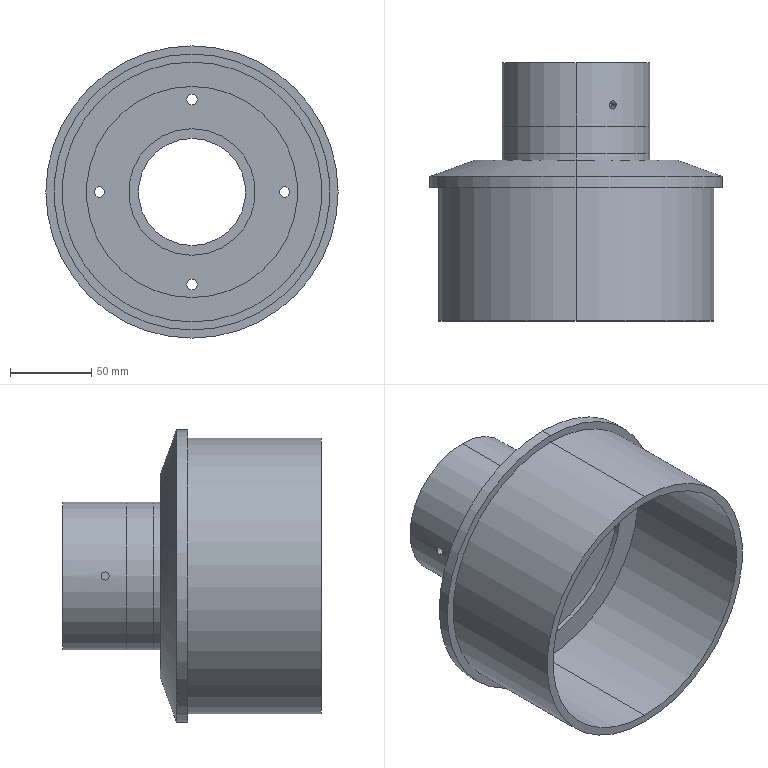Part | SolidWorks | features BaseBody 4 | 4 solids | 85 faces | box 180 x 159.011 x 180 mm | volume 532687 mm3 | cylinder 60 | plane 23 | cone 2 | commonest cylinder face diameters 6.5 x8 10.5 x8 5 x6 78 x6 91 x6 66 x2